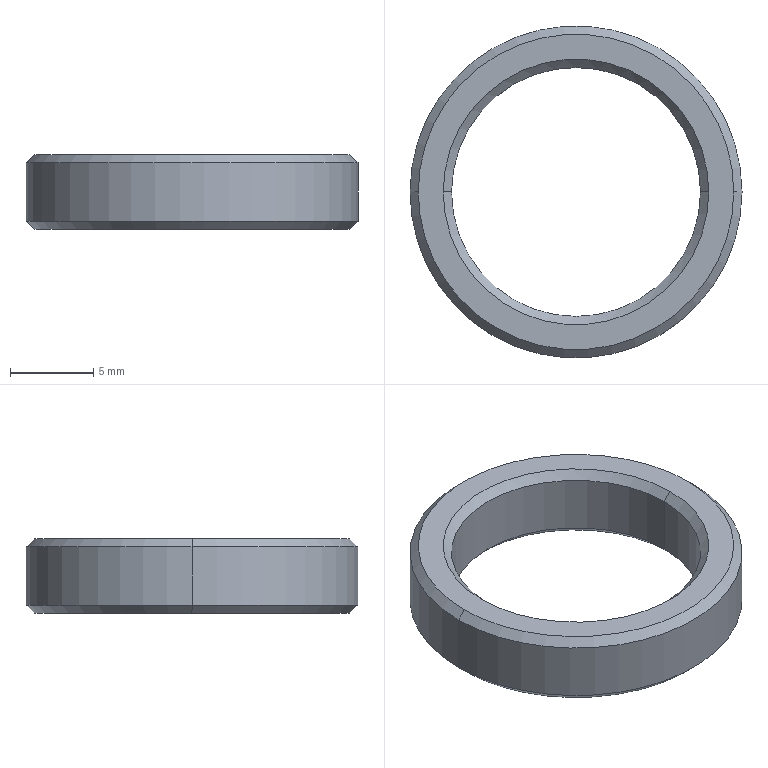Part | SolidWorks | features Chamfer 1, Extrusion 1 | 1 solid | 14 faces | box 20 x 20 x 4.5 mm | volume 591.012 mm3 | cone 8 | cylinder 4 | plane 2 | commonest cylinder face diameters 15 x2 20 x2
STEP:
#1=CARTESIAN_POINT('',(9.5,0.,4.5));
#2=VERTEX_POINT('',#1);
#3=CARTESIAN_POINT('',(-9.5,0.,4.5));
#4=VERTEX_POINT('',#3);
#5=CARTESIAN_POINT('',(0.,0.,4.5));
#6=DIRECTION('',(0.,0.,1.));
#7=DIRECTION('',(1.,0.,0.));
#8=AXIS2_PLACEMENT_3D('',#5,#6,#7);
#9=CIRCLE('',#8,9.5);
#10=EDGE_CURVE('',#2,#4,#9,.T.);
#11=ORIENTED_EDGE('',*,*,#10,.F.);
#12=CARTESIAN_POINT('',(10.,0.,4.));
#13=VERTEX_POINT('',#12);
#14=CARTESIAN_POINT('',(9.5,0.,4.5));
#15=DIRECTION('',(0.7071,0.,-0.7071));
#16=VECTOR('',#15,1000.);
#17=LINE('',#14,#16);
#18=EDGE_CURVE('',#2,#13,#17,.T.);
#19=ORIENTED_EDGE('',*,*,#18,.T.);
#20=CARTESIAN_POINT('',(-10.,0.,4.));
#21=VERTEX_POINT('',#20);
#22=CARTESIAN_POINT('',(0.,0.,4.));
#23=DIRECTION('',(0.,0.,-1.));
#24=DIRECTION('',(1.,0.,0.));
#25=AXIS2_PLACEMENT_3D('',#22,#23,#24);
#26=CIRCLE('',#25,10.);
#27=EDGE_CURVE('',#21,#13,#26,.T.);
#28=ORIENTED_EDGE('',*,*,#27,.F.);
#29=CARTESIAN_POINT('',(-9.5,0.,4.5));
#30=DIRECTION('',(-0.7071,0.,-0.7071));
#31=VECTOR('',#30,1000.);
#32=LINE('',#29,#31);
#33=EDGE_CURVE('',#4,#21,#32,.T.);
#34=ORIENTED_EDGE('',*,*,#33,.F.);
#35=EDGE_LOOP('',(#11,#19,#28,#34));
#36=FACE_OUTER_BOUND('',#35,.T.);
#37=CARTESIAN_POINT('',(0.,0.,4.5));
#38=DIRECTION('',(0.,0.,-1.));
#39=DIRECTION('',(-1.,0.,0.));
#40=AXIS2_PLACEMENT_3D('',#37,#38,#39);
#41=CONICAL_SURFACE('',#40,9.5,0.7854);
#42=ADVANCED_FACE('',(#36),#41,.T.);
#43=CARTESIAN_POINT('',(-7.5,0.,4.));
#44=VERTEX_POINT('',#43);
#45=CARTESIAN_POINT('',(7.5,0.,4.));
#46=VERTEX_POINT('',#45);
#47=CARTESIAN_POINT('',(0.,0.,4.));
#48=DIRECTION('',(0.,0.,1.));
#49=DIRECTION('',(1.,0.,0.));
#50=AXIS2_PLACEMENT_3D('',#47,#48,#49);
#51=CIRCLE('',#50,7.5);
#52=EDGE_CURVE('',#44,#46,#51,.T.);
#53=ORIENTED_EDGE('',*,*,#52,.F.);
#54=CARTESIAN_POINT('',(-8.,0.,4.5));
#55=VERTEX_POINT('',#54);
#56=CARTESIAN_POINT('',(-7.5,0.,4.));
#57=DIRECTION('',(-0.7071,0.,0.7071));
#58=VECTOR('',#57,1000.);
#59=LINE('',#56,#58);
#60=EDGE_CURVE('',#44,#55,#59,.T.);
#61=ORIENTED_EDGE('',*,*,#60,.T.);
#62=CARTESIAN_POINT('',(8.,0.,4.5));
#63=VERTEX_POINT('',#62);
#64=CARTESIAN_POINT('',(0.,0.,4.5));
#65=DIRECTION('',(0.,0.,-1.));
#66=DIRECTION('',(1.,0.,0.));
#67=AXIS2_PLACEMENT_3D('',#64,#65,#66);
#68=CIRCLE('',#67,8.);
#69=EDGE_CURVE('',#63,#55,#68,.T.);
#70=ORIENTED_EDGE('',*,*,#69,.F.);
#71=CARTESIAN_POINT('',(7.5,0.,4.));
#72=DIRECTION('',(0.7071,0.,0.7071));
#73=VECTOR('',#72,1000.);
#74=LINE('',#71,#73);
#75=EDGE_CURVE('',#46,#63,#74,.T.);
#76=ORIENTED_EDGE('',*,*,#75,.F.);
#77=EDGE_LOOP('',(#53,#61,#70,#76));
#78=FACE_OUTER_BOUND('',#77,.T.);
#79=CARTESIAN_POINT('',(0.,0.,4.));
#80=DIRECTION('',(0.,0.,1.));
#81=DIRECTION('',(1.,0.,0.));
#82=AXIS2_PLACEMENT_3D('',#79,#80,#81);
#83=CONICAL_SURFACE('',#82,7.5,0.7854);
#84=ADVANCED_FACE('',(#78),#83,.F.);
#85=CARTESIAN_POINT('',(-9.5,0.,0.));
#86=VERTEX_POINT('',#85);
#87=CARTESIAN_POINT('',(9.5,0.,0.));
#88=VERTEX_POINT('',#87);
#89=CARTESIAN_POINT('',(0.,0.,0.));
#90=DIRECTION('',(0.,0.,-1.));
#91=DIRECTION('',(1.,0.,0.));
#92=AXIS2_PLACEMENT_3D('',#89,#90,#91);
#93=CIRCLE('',#92,9.5);
#94=EDGE_CURVE('',#86,#88,#93,.T.);
#95=ORIENTED_EDGE('',*,*,#94,.F.);
#96=CARTESIAN_POINT('',(-10.,0.,0.5));
#97=VERTEX_POINT('',#96);
#98=CARTESIAN_POINT('',(-10.,0.,0.5));
#99=DIRECTION('',(-0.7071,0.,0.7071));
#100=VECTOR('',#99,1000.);
#101=LINE('',#98,#100);
#102=EDGE_CURVE('',#86,#97,#101,.T.);
#103=ORIENTED_EDGE('',*,*,#102,.T.);
#104=CARTESIAN_POINT('',(10.,0.,0.5));
#105=VERTEX_POINT('',#104);
#106=CARTESIAN_POINT('',(0.,0.,0.5));
#107=DIRECTION('',(0.,0.,1.));
#108=DIRECTION('',(1.,0.,0.));
#109=AXIS2_PLACEMENT_3D('',#106,#107,#108);
#110=CIRCLE('',#109,10.);
#111=EDGE_CURVE('',#105,#97,#110,.T.);
#112=ORIENTED_EDGE('',*,*,#111,.F.);
#113=CARTESIAN_POINT('',(10.,0.,0.5));
#114=DIRECTION('',(0.7071,0.,0.7071));
#115=VECTOR('',#114,1000.);
#116=LINE('',#113,#115);
#117=EDGE_CURVE('',#88,#105,#116,.T.);
#118=ORIENTED_EDGE('',*,*,#117,.F.);
#119=EDGE_LOOP('',(#95,#103,#112,#118));
#120=FACE_OUTER_BOUND('',#119,.T.);
#121=CARTESIAN_POINT('',(0.,0.,0.5));
#122=DIRECTION('',(0.,0.,1.));
#123=DIRECTION('',(1.,0.,0.));
#124=AXIS2_PLACEMENT_3D('',#121,#122,#123);
#125=CONICAL_SURFACE('',#124,10.,0.7854);
#126=ADVANCED_FACE('',(#120),#125,.T.);
#127=CARTESIAN_POINT('',(7.5,0.,0.5));
#128=VERTEX_POINT('',#127);
#129=CARTESIAN_POINT('',(-7.5,0.,0.5));
#130=VERTEX_POINT('',#129);
#131=CARTESIAN_POINT('',(0.,0.,0.5));
#132=DIRECTION('',(0.,0.,-1.));
#133=DIRECTION('',(1.,0.,0.));
#134=AXIS2_PLACEMENT_3D('',#131,#132,#133);
#135=CIRCLE('',#134,7.5);
#136=EDGE_CURVE('',#128,#130,#135,.T.);
#137=ORIENTED_EDGE('',*,*,#136,.F.);
#138=CARTESIAN_POINT('',(8.,0.,0.));
#139=VERTEX_POINT('',#138);
#140=CARTESIAN_POINT('',(8.,0.,0.));
#141=DIRECTION('',(0.7071,0.,-0.7071));
#142=VECTOR('',#141,1000.);
#143=LINE('',#140,#142);
#144=EDGE_CURVE('',#128,#139,#143,.T.);
#145=ORIENTED_EDGE('',*,*,#144,.T.);
#146=CARTESIAN_POINT('',(-8.,0.,0.));
#147=VERTEX_POINT('',#146);
#148=CARTESIAN_POINT('',(0.,0.,0.));
#149=DIRECTION('',(0.,0.,1.));
#150=DIRECTION('',(1.,0.,0.));
#151=AXIS2_PLACEMENT_3D('',#148,#149,#150);
#152=CIRCLE('',#151,8.);
#153=EDGE_CURVE('',#147,#139,#152,.T.);
#154=ORIENTED_EDGE('',*,*,#153,.F.);
#155=CARTESIAN_POINT('',(-8.,0.,0.));
#156=DIRECTION('',(-0.7071,0.,-0.7071));
#157=VECTOR('',#156,1000.);
#158=LINE('',#155,#157);
#159=EDGE_CURVE('',#130,#147,#158,.T.);
#160=ORIENTED_EDGE('',*,*,#159,.F.);
#161=EDGE_LOOP('',(#137,#145,#154,#160));
#162=FACE_OUTER_BOUND('',#161,.T.);
#163=CARTESIAN_POINT('',(0.,0.,0.));
#164=DIRECTION('',(0.,0.,-1.));
#165=DIRECTION('',(-1.,0.,0.));
#166=AXIS2_PLACEMENT_3D('',#163,#164,#165);
#167=CONICAL_SURFACE('',#166,8.,0.7854);
#168=ADVANCED_FACE('',(#162),#167,.F.);
#169=ORIENTED_EDGE('',*,*,#52,.T.);
#170=CARTESIAN_POINT('',(7.5,0.,4.5));
#171=DIRECTION('',(0.,0.,-1.));
#172=VECTOR('',#171,1000.);
#173=LINE('',#170,#172);
#174=EDGE_CURVE('',#46,#128,#173,.T.);
#175=ORIENTED_EDGE('',*,*,#174,.T.);
#176=ORIENTED_EDGE('',*,*,#136,.T.);
#177=CARTESIAN_POINT('',(-7.5,0.,4.5));
#178=DIRECTION('',(0.,0.,-1.));
#179=VECTOR('',#178,1000.);
#180=LINE('',#177,#179);
#181=EDGE_CURVE('',#44,#130,#180,.T.);
#182=ORIENTED_EDGE('',*,*,#181,.F.);
#183=EDGE_LOOP('',(#169,#175,#176,#182));
#184=FACE_OUTER_BOUND('',#183,.T.);
#185=CARTESIAN_POINT('',(0.,0.,4.5));
#186=DIRECTION('',(0.,0.,-1.));
#187=DIRECTION('',(-1.,0.,0.));
#188=AXIS2_PLACEMENT_3D('',#185,#186,#187);
#189=CYLINDRICAL_SURFACE('',#188,7.5);
#190=ADVANCED_FACE('',(#184),#189,.F.);
#191=ORIENTED_EDGE('',*,*,#27,.T.);
#192=CARTESIAN_POINT('',(10.,0.,4.5));
#193=DIRECTION('',(0.,0.,-1.));
#194=VECTOR('',#193,1000.);
#195=LINE('',#192,#194);
#196=EDGE_CURVE('',#13,#105,#195,.T.);
#197=ORIENTED_EDGE('',*,*,#196,.T.);
#198=ORIENTED_EDGE('',*,*,#111,.T.);
#199=CARTESIAN_POINT('',(-10.,0.,4.5));
#200=DIRECTION('',(0.,0.,-1.));
#201=VECTOR('',#200,1000.);
#202=LINE('',#199,#201);
#203=EDGE_CURVE('',#21,#97,#202,.T.);
#204=ORIENTED_EDGE('',*,*,#203,.F.);
#205=EDGE_LOOP('',(#191,#197,#198,#204));
#206=FACE_OUTER_BOUND('',#205,.T.);
#207=CARTESIAN_POINT('',(0.,0.,4.5));
#208=DIRECTION('',(0.,0.,-1.));
#209=DIRECTION('',(-1.,0.,0.));
#210=AXIS2_PLACEMENT_3D('',#207,#208,#209);
#211=CYLINDRICAL_SURFACE('',#210,10.);
#212=ADVANCED_FACE('',(#206),#211,.T.);
#213=ORIENTED_EDGE('',*,*,#69,.T.);
#214=CARTESIAN_POINT('',(0.,0.,4.5));
#215=DIRECTION('',(0.,0.,-1.));
#216=DIRECTION('',(1.,0.,0.));
#217=AXIS2_PLACEMENT_3D('',#214,#215,#216);
#218=CIRCLE('',#217,8.);
#219=EDGE_CURVE('',#55,#63,#218,.T.);
#220=ORIENTED_EDGE('',*,*,#219,.T.);
#221=EDGE_LOOP('',(#213,#220));
#222=FACE_BOUND('',#221,.T.);
#223=CARTESIAN_POINT('',(0.,0.,4.5));
#224=DIRECTION('',(0.,0.,1.));
#225=DIRECTION('',(1.,0.,0.));
#226=AXIS2_PLACEMENT_3D('',#223,#224,#225);
#227=CIRCLE('',#226,9.5);
#228=EDGE_CURVE('',#4,#2,#227,.T.);
#229=ORIENTED_EDGE('',*,*,#228,.T.);
#230=ORIENTED_EDGE('',*,*,#10,.T.);
#231=EDGE_LOOP('',(#229,#230));
#232=FACE_OUTER_BOUND('',#231,.T.);
#233=CARTESIAN_POINT('',(0.,0.,4.5));
#234=DIRECTION('',(0.,0.,1.));
#235=DIRECTION('',(1.,0.,0.));
#236=AXIS2_PLACEMENT_3D('',#233,#234,#235);
#237=PLANE('',#236);
#238=ADVANCED_FACE('',(#222,#232),#237,.T.);
#239=ORIENTED_EDGE('',*,*,#153,.T.);
#240=CARTESIAN_POINT('',(0.,0.,0.));
#241=DIRECTION('',(0.,0.,1.));
#242=DIRECTION('',(1.,0.,0.));
#243=AXIS2_PLACEMENT_3D('',#240,#241,#242);
#244=CIRCLE('',#243,8.);
#245=EDGE_CURVE('',#139,#147,#244,.T.);
#246=ORIENTED_EDGE('',*,*,#245,.T.);
#247=EDGE_LOOP('',(#239,#246));
#248=FACE_BOUND('',#247,.T.);
#249=CARTESIAN_POINT('',(0.,0.,0.));
#250=DIRECTION('',(0.,0.,-1.));
#251=DIRECTION('',(1.,0.,0.));
#252=AXIS2_PLACEMENT_3D('',#249,#250,#251);
#253=CIRCLE('',#252,9.5);
#254=EDGE_CURVE('',#88,#86,#253,.T.);
#255=ORIENTED_EDGE('',*,*,#254,.T.);
#256=ORIENTED_EDGE('',*,*,#94,.T.);
#257=EDGE_LOOP('',(#255,#256));
#258=FACE_OUTER_BOUND('',#257,.T.);
#259=CARTESIAN_POINT('',(0.,0.,0.));
#260=DIRECTION('',(0.,0.,1.));
#261=DIRECTION('',(1.,0.,0.));
#262=AXIS2_PLACEMENT_3D('',#259,#260,#261);
#263=PLANE('',#262);
#264=ADVANCED_FACE('',(#248,#258),#263,.F.);
#265=ORIENTED_EDGE('',*,*,#196,.F.);
#266=CARTESIAN_POINT('',(0.,0.,4.));
#267=DIRECTION('',(0.,0.,-1.));
#268=DIRECTION('',(1.,0.,0.));
#269=AXIS2_PLACEMENT_3D('',#266,#267,#268);
#270=CIRCLE('',#269,10.);
#271=EDGE_CURVE('',#13,#21,#270,.T.);
#272=ORIENTED_EDGE('',*,*,#271,.T.);
#273=ORIENTED_EDGE('',*,*,#203,.T.);
#274=CARTESIAN_POINT('',(0.,0.,0.5));
#275=DIRECTION('',(0.,0.,1.));
#276=DIRECTION('',(1.,0.,0.));
#277=AXIS2_PLACEMENT_3D('',#274,#275,#276);
#278=CIRCLE('',#277,10.);
#279=EDGE_CURVE('',#97,#105,#278,.T.);
#280=ORIENTED_EDGE('',*,*,#279,.T.);
#281=EDGE_LOOP('',(#265,#272,#273,#280));
#282=FACE_OUTER_BOUND('',#281,.T.);
#283=CARTESIAN_POINT('',(0.,0.,4.5));
#284=DIRECTION('',(0.,0.,-1.));
#285=DIRECTION('',(-1.,0.,0.));
#286=AXIS2_PLACEMENT_3D('',#283,#284,#285);
#287=CYLINDRICAL_SURFACE('',#286,10.);
#288=ADVANCED_FACE('',(#282),#287,.T.);
#289=ORIENTED_EDGE('',*,*,#174,.F.);
#290=CARTESIAN_POINT('',(0.,0.,4.));
#291=DIRECTION('',(0.,0.,1.));
#292=DIRECTION('',(1.,0.,0.));
#293=AXIS2_PLACEMENT_3D('',#290,#291,#292);
#294=CIRCLE('',#293,7.5);
#295=EDGE_CURVE('',#46,#44,#294,.T.);
#296=ORIENTED_EDGE('',*,*,#295,.T.);
#297=ORIENTED_EDGE('',*,*,#181,.T.);
#298=CARTESIAN_POINT('',(0.,0.,0.5));
#299=DIRECTION('',(0.,0.,-1.));
#300=DIRECTION('',(1.,0.,0.));
#301=AXIS2_PLACEMENT_3D('',#298,#299,#300);
#302=CIRCLE('',#301,7.5);
#303=EDGE_CURVE('',#130,#128,#302,.T.);
#304=ORIENTED_EDGE('',*,*,#303,.T.);
#305=EDGE_LOOP('',(#289,#296,#297,#304));
#306=FACE_OUTER_BOUND('',#305,.T.);
#307=CARTESIAN_POINT('',(0.,0.,4.5));
#308=DIRECTION('',(0.,0.,-1.));
#309=DIRECTION('',(-1.,0.,0.));
#310=AXIS2_PLACEMENT_3D('',#307,#308,#309);
#311=CYLINDRICAL_SURFACE('',#310,7.5);
#312=ADVANCED_FACE('',(#306),#311,.F.);
#313=ORIENTED_EDGE('',*,*,#144,.F.);
#314=ORIENTED_EDGE('',*,*,#303,.F.);
#315=ORIENTED_EDGE('',*,*,#159,.T.);
#316=ORIENTED_EDGE('',*,*,#245,.F.);
#317=EDGE_LOOP('',(#313,#314,#315,#316));
#318=FACE_OUTER_BOUND('',#317,.T.);
#319=CARTESIAN_POINT('',(0.,0.,0.));
#320=DIRECTION('',(0.,0.,-1.));
#321=DIRECTION('',(-1.,0.,0.));
#322=AXIS2_PLACEMENT_3D('',#319,#320,#321);
#323=CONICAL_SURFACE('',#322,8.,0.7854);
#324=ADVANCED_FACE('',(#318),#323,.F.);
#325=ORIENTED_EDGE('',*,*,#102,.F.);
#326=ORIENTED_EDGE('',*,*,#254,.F.);
#327=ORIENTED_EDGE('',*,*,#117,.T.);
#328=ORIENTED_EDGE('',*,*,#279,.F.);
#329=EDGE_LOOP('',(#325,#326,#327,#328));
#330=FACE_OUTER_BOUND('',#329,.T.);
#331=CARTESIAN_POINT('',(0.,0.,0.5));
#332=DIRECTION('',(0.,0.,1.));
#333=DIRECTION('',(1.,0.,0.));
#334=AXIS2_PLACEMENT_3D('',#331,#332,#333);
#335=CONICAL_SURFACE('',#334,10.,0.7854);
#336=ADVANCED_FACE('',(#330),#335,.T.);
#337=ORIENTED_EDGE('',*,*,#60,.F.);
#338=ORIENTED_EDGE('',*,*,#295,.F.);
#339=ORIENTED_EDGE('',*,*,#75,.T.);
#340=ORIENTED_EDGE('',*,*,#219,.F.);
#341=EDGE_LOOP('',(#337,#338,#339,#340));
#342=FACE_OUTER_BOUND('',#341,.T.);
#343=CARTESIAN_POINT('',(0.,0.,4.));
#344=DIRECTION('',(0.,0.,1.));
#345=DIRECTION('',(1.,0.,0.));
#346=AXIS2_PLACEMENT_3D('',#343,#344,#345);
#347=CONICAL_SURFACE('',#346,7.5,0.7854);
#348=ADVANCED_FACE('',(#342),#347,.F.);
#349=ORIENTED_EDGE('',*,*,#18,.F.);
#350=ORIENTED_EDGE('',*,*,#228,.F.);
#351=ORIENTED_EDGE('',*,*,#33,.T.);
#352=ORIENTED_EDGE('',*,*,#271,.F.);
#353=EDGE_LOOP('',(#349,#350,#351,#352));
#354=FACE_OUTER_BOUND('',#353,.T.);
#355=CARTESIAN_POINT('',(0.,0.,4.5));
#356=DIRECTION('',(0.,0.,-1.));
#357=DIRECTION('',(-1.,0.,0.));
#358=AXIS2_PLACEMENT_3D('',#355,#356,#357);
#359=CONICAL_SURFACE('',#358,9.5,0.7854);
#360=ADVANCED_FACE('',(#354),#359,.T.);
#361=CLOSED_SHELL('',(#42,#84,#126,#168,#190,#212,#238,#264,#288,#312,#324,#336,#348,#360));
#362=MANIFOLD_SOLID_BREP('',#361);
#363=CARTESIAN_POINT('',(0.,0.,0.));
#364=DIRECTION('',(0.,0.,1.));
#365=DIRECTION('',(1.,0.,0.));
#366=AXIS2_PLACEMENT_3D('',#363,#364,#365);
#367=(LENGTH_UNIT()NAMED_UNIT(*)SI_UNIT(.MILLI.,.METRE.));
#368=UNCERTAINTY_MEASURE_WITH_UNIT(LENGTH_MEASURE(0.00001),#367,'','');
#369=(NAMED_UNIT(*)PLANE_ANGLE_UNIT()SI_UNIT($,.RADIAN.));
#370=(NAMED_UNIT(*)SI_UNIT($,.STERADIAN.)SOLID_ANGLE_UNIT());
#371=(GEOMETRIC_REPRESENTATION_CONTEXT(3)GLOBAL_UNCERTAINTY_ASSIGNED_CONTEXT((#368))GLOBAL_UNIT_ASSIGNED_CONTEXT((#367,#369,#370))REPRESENTATION_CONTEXT('',''));
#372=ADVANCED_BREP_SHAPE_REPRESENTATION('',(#362,#366),#371);